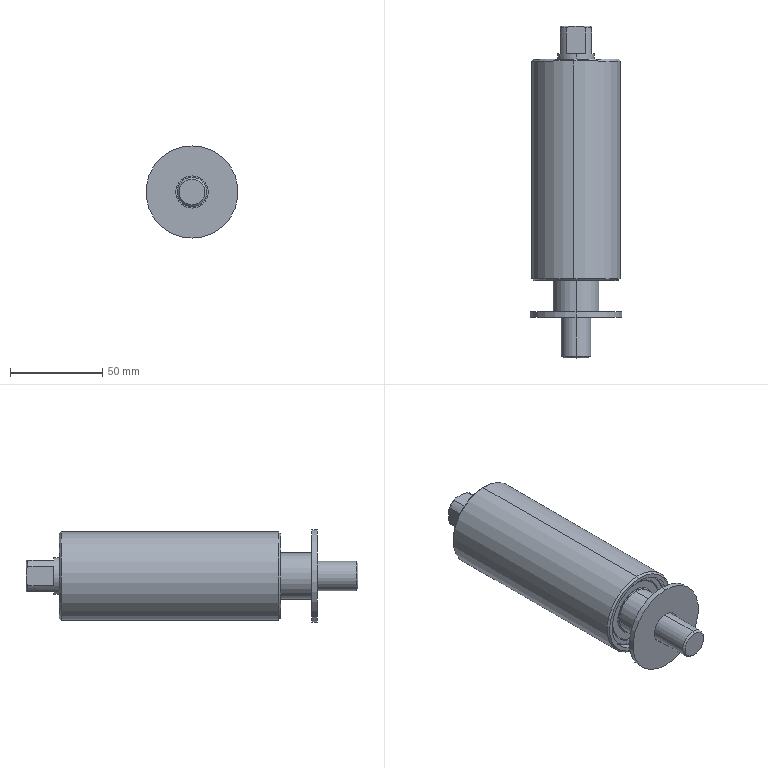Part | SolidWorks | features AEMSimFeature 1 | 35 solids | 424 faces | box 50 x 180 x 50 mm | volume 169491 mm3 | cylinder 162 | sphere 120 | plane 88 | torus 40 | cone 14 | commonest cylinder face diameters 29.9 x54 32.1 x54 20 x8 27.333 x8 34.667 x8 42 x8